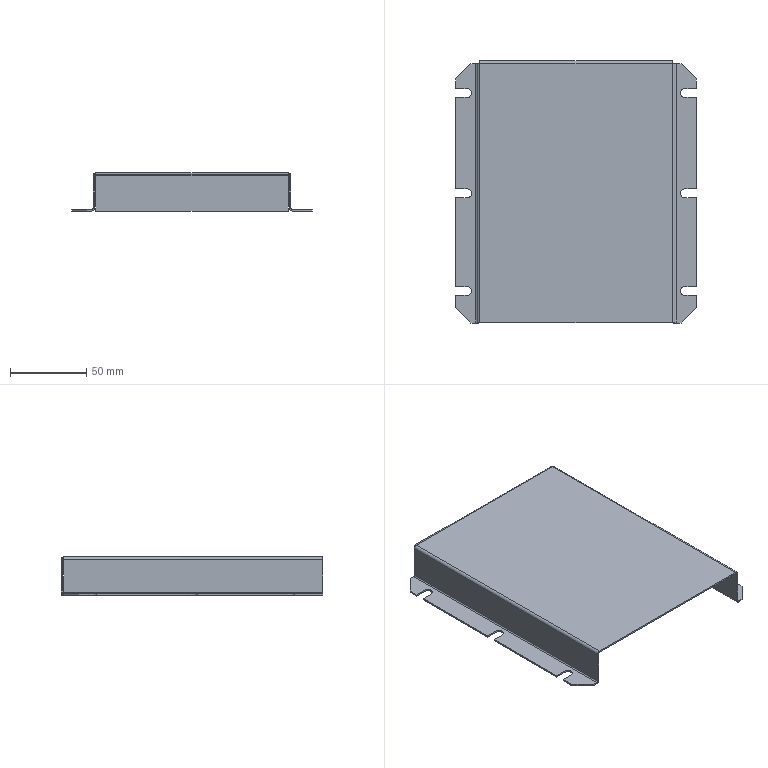Part | SolidWorks | features EdgeFlange 2, BreakCorner 1, FlatPattern 1, HoleWzd 1, SMBaseFlange 1, SheetMetal 1 | 1 solid | 77 faces | box 158 x 172 x 25 mm | volume 37365 mm3 | plane 54 | cylinder 19 | spline 4 | commonest cylinder face diameters 5.8 x9 1.473 x5 3.473 x5